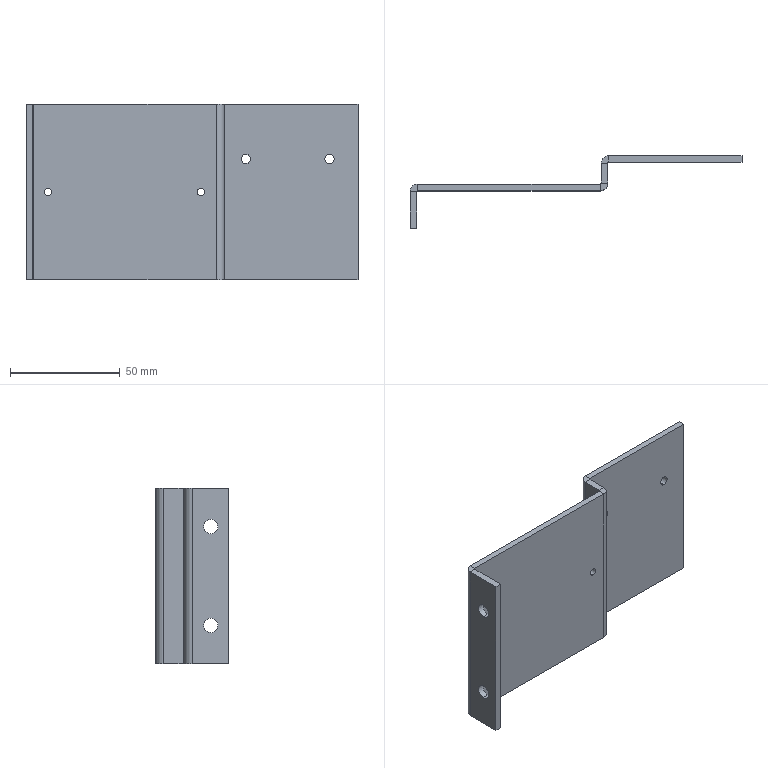Part | SolidWorks | features EdgeFlange 3, HoleWzd 3, FlatPattern 1, SMBaseFlange 1, SheetMetal 1 | 1 solid | 42 faces | box 151 x 33 x 80 mm | volume 42488 mm3 | plane 24 | cylinder 18 | commonest cylinder face diameters 3.3 x4 4.2 x4 6.5 x4 1 x3 7 x3
STEP:
#1=CARTESIAN_POINT('',(55.,13.,17.1));
#2=VERTEX_POINT('',#1);
#3=CARTESIAN_POINT('',(55.,13.,12.9));
#4=VERTEX_POINT('',#3);
#5=CARTESIAN_POINT('',(55.,13.,15.));
#6=DIRECTION('',(0.,-1.,0.));
#7=DIRECTION('',(0.,0.,-1.));
#8=AXIS2_PLACEMENT_3D('',#5,#6,#7);
#9=CIRCLE('',#8,2.1);
#10=EDGE_CURVE('',#2,#4,#9,.T.);
#11=ORIENTED_EDGE('',*,*,#10,.F.);
#12=CARTESIAN_POINT('',(55.,10.,17.1));
#13=VERTEX_POINT('',#12);
#14=CARTESIAN_POINT('',(55.,10.,17.1));
#15=DIRECTION('',(0.,-1.,0.));
#16=VECTOR('',#15,1000.);
#17=LINE('',#14,#16);
#18=EDGE_CURVE('',#2,#13,#17,.T.);
#19=ORIENTED_EDGE('',*,*,#18,.T.);
#20=CARTESIAN_POINT('',(55.,10.,12.9));
#21=VERTEX_POINT('',#20);
#22=CARTESIAN_POINT('',(55.,10.,15.));
#23=DIRECTION('',(0.,-1.,0.));
#24=DIRECTION('',(0.,0.,-1.));
#25=AXIS2_PLACEMENT_3D('',#22,#23,#24);
#26=CIRCLE('',#25,2.1);
#27=EDGE_CURVE('',#13,#21,#26,.T.);
#28=ORIENTED_EDGE('',*,*,#27,.T.);
#29=CARTESIAN_POINT('',(55.,10.,12.9));
#30=DIRECTION('',(0.,-1.,0.));
#31=VECTOR('',#30,1000.);
#32=LINE('',#29,#31);
#33=EDGE_CURVE('',#4,#21,#32,.T.);
#34=ORIENTED_EDGE('',*,*,#33,.F.);
#35=EDGE_LOOP('',(#11,#19,#28,#34));
#36=FACE_OUTER_BOUND('',#35,.T.);
#37=CARTESIAN_POINT('',(55.,10.,15.));
#38=DIRECTION('',(0.,-1.,0.));
#39=DIRECTION('',(0.,0.,-1.));
#40=AXIS2_PLACEMENT_3D('',#37,#38,#39);
#41=CYLINDRICAL_SURFACE('',#40,2.1);
#42=ADVANCED_FACE('',(#36),#41,.F.);
#43=CARTESIAN_POINT('',(93.,13.,17.1));
#44=VERTEX_POINT('',#43);
#45=CARTESIAN_POINT('',(93.,13.,12.9));
#46=VERTEX_POINT('',#45);
#47=CARTESIAN_POINT('',(93.,13.,15.));
#48=DIRECTION('',(0.,-1.,0.));
#49=DIRECTION('',(0.,0.,-1.));
#50=AXIS2_PLACEMENT_3D('',#47,#48,#49);
#51=CIRCLE('',#50,2.1);
#52=EDGE_CURVE('',#44,#46,#51,.T.);
#53=ORIENTED_EDGE('',*,*,#52,.F.);
#54=CARTESIAN_POINT('',(93.,10.,17.1));
#55=VERTEX_POINT('',#54);
#56=CARTESIAN_POINT('',(93.,10.,17.1));
#57=DIRECTION('',(0.,-1.,0.));
#58=VECTOR('',#57,1000.);
#59=LINE('',#56,#58);
#60=EDGE_CURVE('',#44,#55,#59,.T.);
#61=ORIENTED_EDGE('',*,*,#60,.T.);
#62=CARTESIAN_POINT('',(93.,10.,12.9));
#63=VERTEX_POINT('',#62);
#64=CARTESIAN_POINT('',(93.,10.,15.));
#65=DIRECTION('',(0.,-1.,0.));
#66=DIRECTION('',(0.,0.,-1.));
#67=AXIS2_PLACEMENT_3D('',#64,#65,#66);
#68=CIRCLE('',#67,2.1);
#69=EDGE_CURVE('',#55,#63,#68,.T.);
#70=ORIENTED_EDGE('',*,*,#69,.T.);
#71=CARTESIAN_POINT('',(93.,10.,12.9));
#72=DIRECTION('',(0.,-1.,0.));
#73=VECTOR('',#72,1000.);
#74=LINE('',#71,#73);
#75=EDGE_CURVE('',#46,#63,#74,.T.);
#76=ORIENTED_EDGE('',*,*,#75,.F.);
#77=EDGE_LOOP('',(#53,#61,#70,#76));
#78=FACE_OUTER_BOUND('',#77,.T.);
#79=CARTESIAN_POINT('',(93.,10.,15.));
#80=DIRECTION('',(0.,-1.,0.));
#81=DIRECTION('',(0.,0.,-1.));
#82=AXIS2_PLACEMENT_3D('',#79,#80,#81);
#83=CYLINDRICAL_SURFACE('',#82,2.1);
#84=ADVANCED_FACE('',(#78),#83,.F.);
#85=CARTESIAN_POINT('',(-45.,-12.,25.75));
#86=VERTEX_POINT('',#85);
#87=CARTESIAN_POINT('',(-45.,-12.,19.25));
#88=VERTEX_POINT('',#87);
#89=CARTESIAN_POINT('',(-45.,-12.,22.5));
#90=DIRECTION('',(1.,0.,0.));
#91=DIRECTION('',(0.,0.,-1.));
#92=AXIS2_PLACEMENT_3D('',#89,#90,#91);
#93=CIRCLE('',#92,3.25);
#94=EDGE_CURVE('',#86,#88,#93,.T.);
#95=ORIENTED_EDGE('',*,*,#94,.F.);
#96=CARTESIAN_POINT('',(-42.,-12.,25.75));
#97=VERTEX_POINT('',#96);
#98=CARTESIAN_POINT('',(-42.,-12.,25.75));
#99=DIRECTION('',(1.,0.,0.));
#100=VECTOR('',#99,1000.);
#101=LINE('',#98,#100);
#102=EDGE_CURVE('',#86,#97,#101,.T.);
#103=ORIENTED_EDGE('',*,*,#102,.T.);
#104=CARTESIAN_POINT('',(-42.,-12.,19.25));
#105=VERTEX_POINT('',#104);
#106=CARTESIAN_POINT('',(-42.,-12.,22.5));
#107=DIRECTION('',(1.,0.,0.));
#108=DIRECTION('',(0.,0.,-1.));
#109=AXIS2_PLACEMENT_3D('',#106,#107,#108);
#110=CIRCLE('',#109,3.25);
#111=EDGE_CURVE('',#97,#105,#110,.T.);
#112=ORIENTED_EDGE('',*,*,#111,.T.);
#113=CARTESIAN_POINT('',(-42.,-12.,19.25));
#114=DIRECTION('',(1.,0.,0.));
#115=VECTOR('',#114,1000.);
#116=LINE('',#113,#115);
#117=EDGE_CURVE('',#88,#105,#116,.T.);
#118=ORIENTED_EDGE('',*,*,#117,.F.);
#119=EDGE_LOOP('',(#95,#103,#112,#118));
#120=FACE_OUTER_BOUND('',#119,.T.);
#121=CARTESIAN_POINT('',(-42.,-12.,22.5));
#122=DIRECTION('',(1.,0.,0.));
#123=DIRECTION('',(0.,0.,-1.));
#124=AXIS2_PLACEMENT_3D('',#121,#122,#123);
#125=CYLINDRICAL_SURFACE('',#124,3.25);
#126=ADVANCED_FACE('',(#120),#125,.F.);
#127=CARTESIAN_POINT('',(-45.,-12.,-19.25));
#128=VERTEX_POINT('',#127);
#129=CARTESIAN_POINT('',(-45.,-12.,-25.75));
#130=VERTEX_POINT('',#129);
#131=CARTESIAN_POINT('',(-45.,-12.,-22.5));
#132=DIRECTION('',(1.,0.,0.));
#133=DIRECTION('',(0.,0.,-1.));
#134=AXIS2_PLACEMENT_3D('',#131,#132,#133);
#135=CIRCLE('',#134,3.25);
#136=EDGE_CURVE('',#128,#130,#135,.T.);
#137=ORIENTED_EDGE('',*,*,#136,.F.);
#138=CARTESIAN_POINT('',(-42.,-12.,-19.25));
#139=VERTEX_POINT('',#138);
#140=CARTESIAN_POINT('',(-42.,-12.,-19.25));
#141=DIRECTION('',(1.,0.,0.));
#142=VECTOR('',#141,1000.);
#143=LINE('',#140,#142);
#144=EDGE_CURVE('',#128,#139,#143,.T.);
#145=ORIENTED_EDGE('',*,*,#144,.T.);
#146=CARTESIAN_POINT('',(-42.,-12.,-25.75));
#147=VERTEX_POINT('',#146);
#148=CARTESIAN_POINT('',(-42.,-12.,-22.5));
#149=DIRECTION('',(1.,0.,0.));
#150=DIRECTION('',(0.,0.,-1.));
#151=AXIS2_PLACEMENT_3D('',#148,#149,#150);
#152=CIRCLE('',#151,3.25);
#153=EDGE_CURVE('',#139,#147,#152,.T.);
#154=ORIENTED_EDGE('',*,*,#153,.T.);
#155=CARTESIAN_POINT('',(-42.,-12.,-25.75));
#156=DIRECTION('',(1.,0.,0.));
#157=VECTOR('',#156,1000.);
#158=LINE('',#155,#157);
#159=EDGE_CURVE('',#130,#147,#158,.T.);
#160=ORIENTED_EDGE('',*,*,#159,.F.);
#161=EDGE_LOOP('',(#137,#145,#154,#160));
#162=FACE_OUTER_BOUND('',#161,.T.);
#163=CARTESIAN_POINT('',(-42.,-12.,-22.5));
#164=DIRECTION('',(1.,0.,0.));
#165=DIRECTION('',(0.,0.,-1.));
#166=AXIS2_PLACEMENT_3D('',#163,#164,#165);
#167=CYLINDRICAL_SURFACE('',#166,3.25);
#168=ADVANCED_FACE('',(#162),#167,.F.);
#169=CARTESIAN_POINT('',(-35.,-3.,-1.65));
#170=VERTEX_POINT('',#169);
#171=CARTESIAN_POINT('',(-35.,-3.,1.65));
#172=VERTEX_POINT('',#171);
#173=CARTESIAN_POINT('',(-35.,-3.,0.));
#174=DIRECTION('',(0.,1.,0.));
#175=DIRECTION('',(0.,0.,1.));
#176=AXIS2_PLACEMENT_3D('',#173,#174,#175);
#177=CIRCLE('',#176,1.65);
#178=EDGE_CURVE('',#170,#172,#177,.T.);
#179=ORIENTED_EDGE('',*,*,#178,.F.);
#180=CARTESIAN_POINT('',(-35.,0.,-1.65));
#181=VERTEX_POINT('',#180);
#182=CARTESIAN_POINT('',(-35.,0.,-1.65));
#183=DIRECTION('',(0.,1.,0.));
#184=VECTOR('',#183,1000.);
#185=LINE('',#182,#184);
#186=EDGE_CURVE('',#170,#181,#185,.T.);
#187=ORIENTED_EDGE('',*,*,#186,.T.);
#188=CARTESIAN_POINT('',(-35.,0.,1.65));
#189=VERTEX_POINT('',#188);
#190=CARTESIAN_POINT('',(-35.,0.,0.));
#191=DIRECTION('',(0.,1.,0.));
#192=DIRECTION('',(0.,0.,1.));
#193=AXIS2_PLACEMENT_3D('',#190,#191,#192);
#194=CIRCLE('',#193,1.65);
#195=EDGE_CURVE('',#181,#189,#194,.T.);
#196=ORIENTED_EDGE('',*,*,#195,.T.);
#197=CARTESIAN_POINT('',(-35.,0.,1.65));
#198=DIRECTION('',(0.,1.,0.));
#199=VECTOR('',#198,1000.);
#200=LINE('',#197,#199);
#201=EDGE_CURVE('',#172,#189,#200,.T.);
#202=ORIENTED_EDGE('',*,*,#201,.F.);
#203=EDGE_LOOP('',(#179,#187,#196,#202));
#204=FACE_OUTER_BOUND('',#203,.T.);
#205=CARTESIAN_POINT('',(-35.,0.,0.));
#206=DIRECTION('',(0.,1.,0.));
#207=DIRECTION('',(0.,0.,1.));
#208=AXIS2_PLACEMENT_3D('',#205,#206,#207);
#209=CYLINDRICAL_SURFACE('',#208,1.65);
#210=ADVANCED_FACE('',(#204),#209,.F.);
#211=CARTESIAN_POINT('',(34.46,-3.,-1.65));
#212=VERTEX_POINT('',#211);
#213=CARTESIAN_POINT('',(34.46,-3.,1.65));
#214=VERTEX_POINT('',#213);
#215=CARTESIAN_POINT('',(34.46,-3.,0.));
#216=DIRECTION('',(0.,1.,0.));
#217=DIRECTION('',(0.,0.,1.));
#218=AXIS2_PLACEMENT_3D('',#215,#216,#217);
#219=CIRCLE('',#218,1.65);
#220=EDGE_CURVE('',#212,#214,#219,.T.);
#221=ORIENTED_EDGE('',*,*,#220,.F.);
#222=CARTESIAN_POINT('',(34.46,0.,-1.65));
#223=VERTEX_POINT('',#222);
#224=CARTESIAN_POINT('',(34.46,0.,-1.65));
#225=DIRECTION('',(0.,1.,0.));
#226=VECTOR('',#225,1000.);
#227=LINE('',#224,#226);
#228=EDGE_CURVE('',#212,#223,#227,.T.);
#229=ORIENTED_EDGE('',*,*,#228,.T.);
#230=CARTESIAN_POINT('',(34.46,0.,1.65));
#231=VERTEX_POINT('',#230);
#232=CARTESIAN_POINT('',(34.46,0.,0.));
#233=DIRECTION('',(0.,1.,0.));
#234=DIRECTION('',(0.,0.,1.));
#235=AXIS2_PLACEMENT_3D('',#232,#233,#234);
#236=CIRCLE('',#235,1.65);
#237=EDGE_CURVE('',#223,#231,#236,.T.);
#238=ORIENTED_EDGE('',*,*,#237,.T.);
#239=CARTESIAN_POINT('',(34.46,0.,1.65));
#240=DIRECTION('',(0.,1.,0.));
#241=VECTOR('',#240,1000.);
#242=LINE('',#239,#241);
#243=EDGE_CURVE('',#214,#231,#242,.T.);
#244=ORIENTED_EDGE('',*,*,#243,.F.);
#245=EDGE_LOOP('',(#221,#229,#238,#244));
#246=FACE_OUTER_BOUND('',#245,.T.);
#247=CARTESIAN_POINT('',(34.46,0.,0.));
#248=DIRECTION('',(0.,1.,0.));
#249=DIRECTION('',(0.,0.,1.));
#250=AXIS2_PLACEMENT_3D('',#247,#248,#249);
#251=CYLINDRICAL_SURFACE('',#250,1.65);
#252=ADVANCED_FACE('',(#246),#251,.F.);
#253=CARTESIAN_POINT('',(34.46,-3.,0.));
#254=DIRECTION('',(0.,1.,0.));
#255=DIRECTION('',(0.,0.,1.));
#256=AXIS2_PLACEMENT_3D('',#253,#254,#255);
#257=CIRCLE('',#256,1.65);
#258=EDGE_CURVE('',#214,#212,#257,.T.);
#259=ORIENTED_EDGE('',*,*,#258,.T.);
#260=ORIENTED_EDGE('',*,*,#220,.T.);
#261=EDGE_LOOP('',(#259,#260));
#262=FACE_BOUND('',#261,.T.);
#263=CARTESIAN_POINT('',(-35.,-3.,0.));
#264=DIRECTION('',(0.,1.,0.));
#265=DIRECTION('',(0.,0.,1.));
#266=AXIS2_PLACEMENT_3D('',#263,#264,#265);
#267=CIRCLE('',#266,1.65);
#268=EDGE_CURVE('',#172,#170,#267,.T.);
#269=ORIENTED_EDGE('',*,*,#268,.T.);
#270=ORIENTED_EDGE('',*,*,#178,.T.);
#271=EDGE_LOOP('',(#269,#270));
#272=FACE_BOUND('',#271,.T.);
#273=CARTESIAN_POINT('',(-41.5,-3.,-40.));
#274=VERTEX_POINT('',#273);
#275=CARTESIAN_POINT('',(-41.5,-3.,40.));
#276=VERTEX_POINT('',#275);
#277=CARTESIAN_POINT('',(-41.5,-3.,-40.));
#278=DIRECTION('',(0.,0.,1.));
#279=VECTOR('',#278,1000.);
#280=LINE('',#277,#279);
#281=EDGE_CURVE('',#274,#276,#280,.T.);
#282=ORIENTED_EDGE('',*,*,#281,.F.);
#283=CARTESIAN_POINT('',(41.5,-3.,-40.));
#284=VERTEX_POINT('',#283);
#285=CARTESIAN_POINT('',(-45.,-3.,-40.));
#286=DIRECTION('',(1.,0.,0.));
#287=VECTOR('',#286,1000.);
#288=LINE('',#285,#287);
#289=EDGE_CURVE('',#274,#284,#288,.T.);
#290=ORIENTED_EDGE('',*,*,#289,.T.);
#291=CARTESIAN_POINT('',(41.5,-3.,40.));
#292=VERTEX_POINT('',#291);
#293=CARTESIAN_POINT('',(41.5,-3.,-40.));
#294=DIRECTION('',(0.,0.,1.));
#295=VECTOR('',#294,1000.);
#296=LINE('',#293,#295);
#297=EDGE_CURVE('',#284,#292,#296,.T.);
#298=ORIENTED_EDGE('',*,*,#297,.T.);
#299=CARTESIAN_POINT('',(-45.,-3.,40.));
#300=DIRECTION('',(1.,0.,0.));
#301=VECTOR('',#300,1000.);
#302=LINE('',#299,#301);
#303=EDGE_CURVE('',#276,#292,#302,.T.);
#304=ORIENTED_EDGE('',*,*,#303,.F.);
#305=EDGE_LOOP('',(#282,#290,#298,#304));
#306=FACE_OUTER_BOUND('',#305,.T.);
#307=CARTESIAN_POINT('',(-45.,-3.,40.));
#308=DIRECTION('',(0.,1.,0.));
#309=DIRECTION('',(-1.,0.,0.));
#310=AXIS2_PLACEMENT_3D('',#307,#308,#309);
#311=PLANE('',#310);
#312=ADVANCED_FACE('',(#262,#272,#306),#311,.F.);
#313=CARTESIAN_POINT('',(-35.,0.,0.));
#314=DIRECTION('',(0.,1.,0.));
#315=DIRECTION('',(0.,0.,1.));
#316=AXIS2_PLACEMENT_3D('',#313,#314,#315);
#317=CIRCLE('',#316,1.65);
#318=EDGE_CURVE('',#189,#181,#317,.T.);
#319=ORIENTED_EDGE('',*,*,#318,.F.);
#320=ORIENTED_EDGE('',*,*,#195,.F.);
#321=EDGE_LOOP('',(#319,#320));
#322=FACE_BOUND('',#321,.T.);
#323=CARTESIAN_POINT('',(34.46,0.,0.));
#324=DIRECTION('',(0.,1.,0.));
#325=DIRECTION('',(0.,0.,1.));
#326=AXIS2_PLACEMENT_3D('',#323,#324,#325);
#327=CIRCLE('',#326,1.65);
#328=EDGE_CURVE('',#231,#223,#327,.T.);
#329=ORIENTED_EDGE('',*,*,#328,.F.);
#330=ORIENTED_EDGE('',*,*,#237,.F.);
#331=EDGE_LOOP('',(#329,#330));
#332=FACE_BOUND('',#331,.T.);
#333=CARTESIAN_POINT('',(-41.5,0.,-40.));
#334=VERTEX_POINT('',#333);
#335=CARTESIAN_POINT('',(41.5,0.,-40.));
#336=VERTEX_POINT('',#335);
#337=CARTESIAN_POINT('',(-45.,0.,-40.));
#338=DIRECTION('',(1.,0.,0.));
#339=VECTOR('',#338,1000.);
#340=LINE('',#337,#339);
#341=EDGE_CURVE('',#334,#336,#340,.T.);
#342=ORIENTED_EDGE('',*,*,#341,.F.);
#343=CARTESIAN_POINT('',(-41.5,0.,40.));
#344=VERTEX_POINT('',#343);
#345=CARTESIAN_POINT('',(-41.5,0.,-40.));
#346=DIRECTION('',(0.,0.,1.));
#347=VECTOR('',#346,1000.);
#348=LINE('',#345,#347);
#349=EDGE_CURVE('',#334,#344,#348,.T.);
#350=ORIENTED_EDGE('',*,*,#349,.T.);
#351=CARTESIAN_POINT('',(41.5,0.,40.));
#352=VERTEX_POINT('',#351);
#353=CARTESIAN_POINT('',(-45.,0.,40.));
#354=DIRECTION('',(1.,0.,0.));
#355=VECTOR('',#354,1000.);
#356=LINE('',#353,#355);
#357=EDGE_CURVE('',#344,#352,#356,.T.);
#358=ORIENTED_EDGE('',*,*,#357,.T.);
#359=CARTESIAN_POINT('',(41.5,0.,-40.));
#360=DIRECTION('',(0.,0.,1.));
#361=VECTOR('',#360,1000.);
#362=LINE('',#359,#361);
#363=EDGE_CURVE('',#336,#352,#362,.T.);
#364=ORIENTED_EDGE('',*,*,#363,.F.);
#365=EDGE_LOOP('',(#342,#350,#358,#364));
#366=FACE_OUTER_BOUND('',#365,.T.);
#367=CARTESIAN_POINT('',(-45.,0.,40.));
#368=DIRECTION('',(0.,1.,0.));
#369=DIRECTION('',(-1.,0.,0.));
#370=AXIS2_PLACEMENT_3D('',#367,#368,#369);
#371=PLANE('',#370);
#372=ADVANCED_FACE('',(#322,#332,#366),#371,.T.);
#373=CARTESIAN_POINT('',(-41.5,-3.,40.));
#374=DIRECTION('',(0.,1.,0.));
#375=VECTOR('',#374,1000.);
#376=LINE('',#373,#375);
#377=EDGE_CURVE('',#276,#344,#376,.T.);
#378=ORIENTED_EDGE('',*,*,#377,.F.);
#379=ORIENTED_EDGE('',*,*,#303,.T.);
#380=CARTESIAN_POINT('',(41.5,0.,40.));
#381=DIRECTION('',(0.,-1.,0.));
#382=VECTOR('',#381,1000.);
#383=LINE('',#380,#382);
#384=EDGE_CURVE('',#352,#292,#383,.T.);
#385=ORIENTED_EDGE('',*,*,#384,.F.);
#386=ORIENTED_EDGE('',*,*,#357,.F.);
#387=EDGE_LOOP('',(#378,#379,#385,#386));
#388=FACE_OUTER_BOUND('',#387,.T.);
#389=CARTESIAN_POINT('',(0.,0.,40.));
#390=DIRECTION('',(0.,0.,-1.));
#391=DIRECTION('',(-1.,0.,0.));
#392=AXIS2_PLACEMENT_3D('',#389,#390,#391);
#393=PLANE('',#392);
#394=ADVANCED_FACE('',(#388),#393,.F.);
#395=ORIENTED_EDGE('',*,*,#289,.F.);
#396=CARTESIAN_POINT('',(-41.5,-3.,-40.));
#397=DIRECTION('',(0.,1.,0.));
#398=VECTOR('',#397,1000.);
#399=LINE('',#396,#398);
#400=EDGE_CURVE('',#274,#334,#399,.T.);
#401=ORIENTED_EDGE('',*,*,#400,.T.);
#402=ORIENTED_EDGE('',*,*,#341,.T.);
#403=CARTESIAN_POINT('',(41.5,0.,-40.));
#404=DIRECTION('',(0.,-1.,0.));
#405=VECTOR('',#404,1000.);
#406=LINE('',#403,#405);
#407=EDGE_CURVE('',#336,#284,#406,.T.);
#408=ORIENTED_EDGE('',*,*,#407,.T.);
#409=EDGE_LOOP('',(#395,#401,#402,#408));
#410=FACE_OUTER_BOUND('',#409,.T.);
#411=CARTESIAN_POINT('',(0.,0.,-40.));
#412=DIRECTION('',(0.,0.,-1.));
#413=DIRECTION('',(-1.,0.,0.));
#414=AXIS2_PLACEMENT_3D('',#411,#412,#413);
#415=PLANE('',#414);
#416=ADVANCED_FACE('',(#410),#415,.T.);
#417=CARTESIAN_POINT('',(45.,9.5,40.));
#418=VERTEX_POINT('',#417);
#419=CARTESIAN_POINT('',(42.,9.5,40.));
#420=VERTEX_POINT('',#419);
#421=CARTESIAN_POINT('',(45.,9.5,40.));
#422=DIRECTION('',(-1.,0.,0.));
#423=VECTOR('',#422,1000.);
#424=LINE('',#421,#423);
#425=EDGE_CURVE('',#418,#420,#424,.T.);
#426=ORIENTED_EDGE('',*,*,#425,.T.);
#427=CARTESIAN_POINT('',(42.,0.5,40.));
#428=VERTEX_POINT('',#427);
#429=CARTESIAN_POINT('',(42.,0.,40.));
#430=DIRECTION('',(0.,-1.,0.));
#431=VECTOR('',#430,1000.);
#432=LINE('',#429,#431);
#433=EDGE_CURVE('',#420,#428,#432,.T.);
#434=ORIENTED_EDGE('',*,*,#433,.T.);
#435=CARTESIAN_POINT('',(45.,0.5,40.));
#436=VERTEX_POINT('',#435);
#437=CARTESIAN_POINT('',(45.,0.5,40.));
#438=DIRECTION('',(1.,0.,0.));
#439=VECTOR('',#438,1000.);
#440=LINE('',#437,#439);
#441=EDGE_CURVE('',#428,#436,#440,.T.);
#442=ORIENTED_EDGE('',*,*,#441,.T.);
#443=CARTESIAN_POINT('',(45.,0.,40.));
#444=DIRECTION('',(0.,-1.,0.));
#445=VECTOR('',#444,1000.);
#446=LINE('',#443,#445);
#447=EDGE_CURVE('',#418,#436,#446,.T.);
#448=ORIENTED_EDGE('',*,*,#447,.F.);
#449=EDGE_LOOP('',(#426,#434,#442,#448));
#450=FACE_OUTER_BOUND('',#449,.T.);
#451=CARTESIAN_POINT('',(45.,0.,40.));
#452=DIRECTION('',(0.,0.,-1.));
#453=DIRECTION('',(-1.,0.,0.));
#454=AXIS2_PLACEMENT_3D('',#451,#452,#453);
#455=PLANE('',#454);
#456=ADVANCED_FACE('',(#450),#455,.F.);
#457=CARTESIAN_POINT('',(45.,9.5,-40.));
#458=VERTEX_POINT('',#457);
#459=CARTESIAN_POINT('',(42.,9.5,-40.));
#460=VERTEX_POINT('',#459);
#461=CARTESIAN_POINT('',(45.,9.5,-40.));
#462=DIRECTION('',(-1.,0.,0.));
#463=VECTOR('',#462,1000.);
#464=LINE('',#461,#463);
#465=EDGE_CURVE('',#458,#460,#464,.T.);
#466=ORIENTED_EDGE('',*,*,#465,.F.);
#467=CARTESIAN_POINT('',(45.,0.5,-40.));
#468=VERTEX_POINT('',#467);
#469=CARTESIAN_POINT('',(45.,0.,-40.));
#470=DIRECTION('',(0.,1.,0.));
#471=VECTOR('',#470,1000.);
#472=LINE('',#469,#471);
#473=EDGE_CURVE('',#468,#458,#472,.T.);
#474=ORIENTED_EDGE('',*,*,#473,.F.);
#475=CARTESIAN_POINT('',(42.,0.5,-40.));
#476=VERTEX_POINT('',#475);
#477=CARTESIAN_POINT('',(42.,0.5,-40.));
#478=DIRECTION('',(1.,0.,0.));
#479=VECTOR('',#478,1000.);
#480=LINE('',#477,#479);
#481=EDGE_CURVE('',#476,#468,#480,.T.);
#482=ORIENTED_EDGE('',*,*,#481,.F.);
#483=CARTESIAN_POINT('',(42.,13.,-40.));
#484=DIRECTION('',(0.,1.,0.));
#485=VECTOR('',#484,1000.);
#486=LINE('',#483,#485);
#487=EDGE_CURVE('',#476,#460,#486,.T.);
#488=ORIENTED_EDGE('',*,*,#487,.T.);
#489=EDGE_LOOP('',(#466,#474,#482,#488));
#490=FACE_OUTER_BOUND('',#489,.T.);
#491=CARTESIAN_POINT('',(45.,13.,-40.));
#492=DIRECTION('',(0.,0.,1.));
#493=DIRECTION('',(0.,-1.,0.));
#494=AXIS2_PLACEMENT_3D('',#491,#492,#493);
#495=PLANE('',#494);
#496=ADVANCED_FACE('',(#490),#495,.F.);
#497=CARTESIAN_POINT('',(45.,9.5,40.));
#498=DIRECTION('',(0.,0.,-1.));
#499=VECTOR('',#498,1000.);
#500=LINE('',#497,#499);
#501=EDGE_CURVE('',#418,#458,#500,.T.);
#502=ORIENTED_EDGE('',*,*,#501,.F.);
#503=ORIENTED_EDGE('',*,*,#447,.T.);
#504=CARTESIAN_POINT('',(45.,0.5,40.));
#505=DIRECTION('',(0.,0.,1.));
#506=VECTOR('',#505,1000.);
#507=LINE('',#504,#506);
#508=EDGE_CURVE('',#468,#436,#507,.T.);
#509=ORIENTED_EDGE('',*,*,#508,.F.);
#510=ORIENTED_EDGE('',*,*,#473,.T.);
#511=EDGE_LOOP('',(#502,#503,#509,#510));
#512=FACE_OUTER_BOUND('',#511,.T.);
#513=CARTESIAN_POINT('',(45.,0.,0.));
#514=DIRECTION('',(-1.,0.,0.));
#515=DIRECTION('',(0.,-1.,0.));
#516=AXIS2_PLACEMENT_3D('',#513,#514,#515);
#517=PLANE('',#516);
#518=ADVANCED_FACE('',(#512),#517,.F.);
#519=ORIENTED_EDGE('',*,*,#433,.F.);
#520=CARTESIAN_POINT('',(42.,9.5,40.));
#521=DIRECTION('',(0.,0.,-1.));
#522=VECTOR('',#521,1000.);
#523=LINE('',#520,#522);
#524=EDGE_CURVE('',#420,#460,#523,.T.);
#525=ORIENTED_EDGE('',*,*,#524,.T.);
#526=ORIENTED_EDGE('',*,*,#487,.F.);
#527=CARTESIAN_POINT('',(42.,0.5,40.));
#528=DIRECTION('',(0.,0.,-1.));
#529=VECTOR('',#528,1000.);
#530=LINE('',#527,#529);
#531=EDGE_CURVE('',#428,#476,#530,.T.);
#532=ORIENTED_EDGE('',*,*,#531,.F.);
#533=EDGE_LOOP('',(#519,#525,#526,#532));
#534=FACE_OUTER_BOUND('',#533,.T.);
#535=CARTESIAN_POINT('',(42.,0.,0.));
#536=DIRECTION('',(-1.,0.,0.));
#537=DIRECTION('',(0.,-1.,0.));
#538=AXIS2_PLACEMENT_3D('',#535,#536,#537);
#539=PLANE('',#538);
#540=ADVANCED_FACE('',(#534),#539,.T.);
#541=ORIENTED_EDGE('',*,*,#441,.F.);
#542=CARTESIAN_POINT('',(41.5,0.5,40.));
#543=DIRECTION('',(0.,0.,1.));
#544=DIRECTION('',(-1.,0.,0.));
#545=AXIS2_PLACEMENT_3D('',#542,#543,#544);
#546=CIRCLE('',#545,0.5);
#547=EDGE_CURVE('',#352,#428,#546,.T.);
#548=ORIENTED_EDGE('',*,*,#547,.F.);
#549=ORIENTED_EDGE('',*,*,#384,.T.);
#550=CARTESIAN_POINT('',(41.5,0.5,40.));
#551=DIRECTION('',(0.,0.,1.));
#552=DIRECTION('',(-1.,0.,0.));
#553=AXIS2_PLACEMENT_3D('',#550,#551,#552);
#554=CIRCLE('',#553,3.5);
#555=EDGE_CURVE('',#292,#436,#554,.T.);
#556=ORIENTED_EDGE('',*,*,#555,.T.);
#557=EDGE_LOOP('',(#541,#548,#549,#556));
#558=FACE_OUTER_BOUND('',#557,.T.);
#559=CARTESIAN_POINT('',(41.5,0.5,40.));
#560=DIRECTION('',(0.,0.,1.));
#561=DIRECTION('',(1.,0.,0.));
#562=AXIS2_PLACEMENT_3D('',#559,#560,#561);
#563=PLANE('',#562);
#564=ADVANCED_FACE('',(#558),#563,.T.);
#565=CARTESIAN_POINT('',(41.5,0.5,-40.));
#566=DIRECTION('',(0.,0.,-1.));
#567=DIRECTION('',(-1.,0.,0.));
#568=AXIS2_PLACEMENT_3D('',#565,#566,#567);
#569=CIRCLE('',#568,0.5);
#570=EDGE_CURVE('',#476,#336,#569,.T.);
#571=ORIENTED_EDGE('',*,*,#570,.F.);
#572=ORIENTED_EDGE('',*,*,#481,.T.);
#573=CARTESIAN_POINT('',(41.5,0.5,-40.));
#574=DIRECTION('',(0.,0.,-1.));
#575=DIRECTION('',(-1.,0.,0.));
#576=AXIS2_PLACEMENT_3D('',#573,#574,#575);
#577=CIRCLE('',#576,3.5);
#578=EDGE_CURVE('',#468,#284,#577,.T.);
#579=ORIENTED_EDGE('',*,*,#578,.T.);
#580=ORIENTED_EDGE('',*,*,#407,.F.);
#581=EDGE_LOOP('',(#571,#572,#579,#580));
#582=FACE_OUTER_BOUND('',#581,.T.);
#583=CARTESIAN_POINT('',(41.5,0.5,-40.));
#584=DIRECTION('',(0.,0.,1.));
#585=DIRECTION('',(1.,0.,0.));
#586=AXIS2_PLACEMENT_3D('',#583,#584,#585);
#587=PLANE('',#586);
#588=ADVANCED_FACE('',(#582),#587,.F.);
#589=ORIENTED_EDGE('',*,*,#297,.F.);
#590=ORIENTED_EDGE('',*,*,#578,.F.);
#591=ORIENTED_EDGE('',*,*,#508,.T.);
#592=ORIENTED_EDGE('',*,*,#555,.F.);
#593=EDGE_LOOP('',(#589,#590,#591,#592));
#594=FACE_OUTER_BOUND('',#593,.T.);
#595=CARTESIAN_POINT('',(41.5,0.5,-40.));
#596=DIRECTION('',(0.,0.,-1.));
#597=DIRECTION('',(1.,0.,0.));
#598=AXIS2_PLACEMENT_3D('',#595,#596,#597);
#599=CYLINDRICAL_SURFACE('',#598,3.5);
#600=ADVANCED_FACE('',(#594),#599,.T.);
#601=ORIENTED_EDGE('',*,*,#363,.T.);
#602=ORIENTED_EDGE('',*,*,#547,.T.);
#603=ORIENTED_EDGE('',*,*,#531,.T.);
#604=ORIENTED_EDGE('',*,*,#570,.T.);
#605=EDGE_LOOP('',(#601,#602,#603,#604));
#606=FACE_OUTER_BOUND('',#605,.T.);
#607=CARTESIAN_POINT('',(41.5,0.5,-40.));
#608=DIRECTION('',(0.,0.,-1.));
#609=DIRECTION('',(1.,0.,0.));
#610=AXIS2_PLACEMENT_3D('',#607,#608,#609);
#611=CYLINDRICAL_SURFACE('',#610,0.5);
#612=ADVANCED_FACE('',(#606),#611,.F.);
#613=CARTESIAN_POINT('',(45.5,10.,-40.));
#614=VERTEX_POINT('',#613);
#615=CARTESIAN_POINT('',(45.5,13.,-40.));
#616=VERTEX_POINT('',#615);
#617=CARTESIAN_POINT('',(45.5,13.,-40.));
#618=DIRECTION('',(0.,1.,0.));
#619=VECTOR('',#618,1000.);
#620=LINE('',#617,#619);
#621=EDGE_CURVE('',#614,#616,#620,.T.);
#622=ORIENTED_EDGE('',*,*,#621,.F.);
#623=CARTESIAN_POINT('',(45.5,9.5,-40.));
#624=DIRECTION('',(0.,0.,-1.));
#625=DIRECTION('',(1.,0.,0.));
#626=AXIS2_PLACEMENT_3D('',#623,#624,#625);
#627=CIRCLE('',#626,0.5);
#628=EDGE_CURVE('',#458,#614,#627,.T.);
#629=ORIENTED_EDGE('',*,*,#628,.F.);
#630=ORIENTED_EDGE('',*,*,#465,.T.);
#631=CARTESIAN_POINT('',(45.5,9.5,-40.));
#632=DIRECTION('',(0.,0.,-1.));
#633=DIRECTION('',(1.,0.,0.));
#634=AXIS2_PLACEMENT_3D('',#631,#632,#633);
#635=CIRCLE('',#634,3.5);
#636=EDGE_CURVE('',#460,#616,#635,.T.);
#637=ORIENTED_EDGE('',*,*,#636,.T.);
#638=EDGE_LOOP('',(#622,#629,#630,#637));
#639=FACE_OUTER_BOUND('',#638,.T.);
#640=CARTESIAN_POINT('',(45.5,9.5,-40.));
#641=DIRECTION('',(0.,0.,-1.));
#642=DIRECTION('',(-1.,0.,0.));
#643=AXIS2_PLACEMENT_3D('',#640,#641,#642);
#644=PLANE('',#643);
#645=ADVANCED_FACE('',(#639),#644,.T.);
#646=CARTESIAN_POINT('',(45.5,10.,40.));
#647=VERTEX_POINT('',#646);
#648=CARTESIAN_POINT('',(45.5,9.5,40.));
#649=DIRECTION('',(0.,0.,1.));
#650=DIRECTION('',(1.,0.,0.));
#651=AXIS2_PLACEMENT_3D('',#648,#649,#650);
#652=CIRCLE('',#651,0.5);
#653=EDGE_CURVE('',#647,#418,#652,.T.);
#654=ORIENTED_EDGE('',*,*,#653,.F.);
#655=CARTESIAN_POINT('',(45.5,13.,40.));
#656=VERTEX_POINT('',#655);
#657=CARTESIAN_POINT('',(45.5,10.,40.));
#658=DIRECTION('',(0.,1.,0.));
#659=VECTOR('',#658,1000.);
#660=LINE('',#657,#659);
#661=EDGE_CURVE('',#647,#656,#660,.T.);
#662=ORIENTED_EDGE('',*,*,#661,.T.);
#663=CARTESIAN_POINT('',(45.5,9.5,40.));
#664=DIRECTION('',(0.,0.,1.));
#665=DIRECTION('',(1.,0.,0.));
#666=AXIS2_PLACEMENT_3D('',#663,#664,#665);
#667=CIRCLE('',#666,3.5);
#668=EDGE_CURVE('',#656,#420,#667,.T.);
#669=ORIENTED_EDGE('',*,*,#668,.T.);
#670=ORIENTED_EDGE('',*,*,#425,.F.);
#671=EDGE_LOOP('',(#654,#662,#669,#670));
#672=FACE_OUTER_BOUND('',#671,.T.);
#673=CARTESIAN_POINT('',(45.5,9.5,40.));
#674=DIRECTION('',(0.,0.,-1.));
#675=DIRECTION('',(-1.,0.,0.));
#676=AXIS2_PLACEMENT_3D('',#673,#674,#675);
#677=PLANE('',#676);
#678=ADVANCED_FACE('',(#672),#677,.F.);
#679=ORIENTED_EDGE('',*,*,#524,.F.);
#680=ORIENTED_EDGE('',*,*,#668,.F.);
#681=CARTESIAN_POINT('',(45.5,13.,-40.));
#682=DIRECTION('',(0.,0.,-1.));
#683=VECTOR('',#682,1000.);
#684=LINE('',#681,#683);
#685=EDGE_CURVE('',#656,#616,#684,.T.);
#686=ORIENTED_EDGE('',*,*,#685,.T.);
#687=ORIENTED_EDGE('',*,*,#636,.F.);
#688=EDGE_LOOP('',(#679,#680,#686,#687));
#689=FACE_OUTER_BOUND('',#688,.T.);
#690=CARTESIAN_POINT('',(45.5,9.5,40.));
#691=DIRECTION('',(0.,0.,1.));
#692=DIRECTION('',(0.,1.,0.));
#693=AXIS2_PLACEMENT_3D('',#690,#691,#692);
#694=CYLINDRICAL_SURFACE('',#693,3.5);
#695=ADVANCED_FACE('',(#689),#694,.T.);
#696=ORIENTED_EDGE('',*,*,#501,.T.);
#697=ORIENTED_EDGE('',*,*,#628,.T.);
#698=CARTESIAN_POINT('',(45.5,10.,-40.));
#699=DIRECTION('',(0.,0.,1.));
#700=VECTOR('',#699,1000.);
#701=LINE('',#698,#700);
#702=EDGE_CURVE('',#614,#647,#701,.T.);
#703=ORIENTED_EDGE('',*,*,#702,.T.);
#704=ORIENTED_EDGE('',*,*,#653,.T.);
#705=EDGE_LOOP('',(#696,#697,#703,#704));
#706=FACE_OUTER_BOUND('',#705,.T.);
#707=CARTESIAN_POINT('',(45.5,9.5,40.));
#708=DIRECTION('',(0.,0.,1.));
#709=DIRECTION('',(0.,1.,0.));
#710=AXIS2_PLACEMENT_3D('',#707,#708,#709);
#711=CYLINDRICAL_SURFACE('',#710,0.5);
#712=ADVANCED_FACE('',(#706),#711,.F.);
#713=ORIENTED_EDGE('',*,*,#621,.T.);
#714=CARTESIAN_POINT('',(106.,13.,-40.));
#715=VERTEX_POINT('',#714);
#716=CARTESIAN_POINT('',(0.,13.,-40.));
#717=DIRECTION('',(-1.,0.,0.));
#718=VECTOR('',#717,1000.);
#719=LINE('',#716,#718);
#720=EDGE_CURVE('',#715,#616,#719,.T.);
#721=ORIENTED_EDGE('',*,*,#720,.F.);
#722=CARTESIAN_POINT('',(106.,10.,-40.));
#723=VERTEX_POINT('',#722);
#724=CARTESIAN_POINT('',(106.,13.,-40.));
#725=DIRECTION('',(0.,-1.,0.));
#726=VECTOR('',#725,1000.);
#727=LINE('',#724,#726);
#728=EDGE_CURVE('',#715,#723,#727,.T.);
#729=ORIENTED_EDGE('',*,*,#728,.T.);
#730=CARTESIAN_POINT('',(45.,10.,-40.));
#731=DIRECTION('',(-1.,0.,0.));
#732=VECTOR('',#731,1000.);
#733=LINE('',#730,#732);
#734=EDGE_CURVE('',#723,#614,#733,.T.);
#735=ORIENTED_EDGE('',*,*,#734,.T.);
#736=EDGE_LOOP('',(#713,#721,#729,#735));
#737=FACE_OUTER_BOUND('',#736,.T.);
#738=CARTESIAN_POINT('',(45.,13.,-40.));
#739=DIRECTION('',(0.,0.,1.));
#740=DIRECTION('',(1.,0.,0.));
#741=AXIS2_PLACEMENT_3D('',#738,#739,#740);
#742=PLANE('',#741);
#743=ADVANCED_FACE('',(#737),#742,.F.);
#744=ORIENTED_EDGE('',*,*,#661,.F.);
#745=CARTESIAN_POINT('',(106.,10.,40.));
#746=VERTEX_POINT('',#745);
#747=CARTESIAN_POINT('',(106.,10.,40.));
#748=DIRECTION('',(1.,0.,0.));
#749=VECTOR('',#748,1000.);
#750=LINE('',#747,#749);
#751=EDGE_CURVE('',#647,#746,#750,.T.);
#752=ORIENTED_EDGE('',*,*,#751,.T.);
#753=CARTESIAN_POINT('',(106.,13.,40.));
#754=VERTEX_POINT('',#753);
#755=CARTESIAN_POINT('',(106.,13.,40.));
#756=DIRECTION('',(0.,-1.,0.));
#757=VECTOR('',#756,1000.);
#758=LINE('',#755,#757);
#759=EDGE_CURVE('',#754,#746,#758,.T.);
#760=ORIENTED_EDGE('',*,*,#759,.F.);
#761=CARTESIAN_POINT('',(0.,13.,40.));
#762=DIRECTION('',(1.,0.,0.));
#763=VECTOR('',#762,1000.);
#764=LINE('',#761,#763);
#765=EDGE_CURVE('',#656,#754,#764,.T.);
#766=ORIENTED_EDGE('',*,*,#765,.F.);
#767=EDGE_LOOP('',(#744,#752,#760,#766));
#768=FACE_OUTER_BOUND('',#767,.T.);
#769=CARTESIAN_POINT('',(106.,13.,40.));
#770=DIRECTION('',(0.,0.,-1.));
#771=DIRECTION('',(-1.,0.,0.));
#772=AXIS2_PLACEMENT_3D('',#769,#770,#771);
#773=PLANE('',#772);
#774=ADVANCED_FACE('',(#768),#773,.F.);
#775=CARTESIAN_POINT('',(55.,13.,15.));
#776=DIRECTION('',(0.,-1.,0.));
#777=DIRECTION('',(0.,0.,-1.));
#778=AXIS2_PLACEMENT_3D('',#775,#776,#777);
#779=CIRCLE('',#778,2.1);
#780=EDGE_CURVE('',#4,#2,#779,.T.);
#781=ORIENTED_EDGE('',*,*,#780,.T.);
#782=ORIENTED_EDGE('',*,*,#10,.T.);
#783=EDGE_LOOP('',(#781,#782));
#784=FACE_BOUND('',#783,.T.);
#785=CARTESIAN_POINT('',(93.,13.,15.));
#786=DIRECTION('',(0.,-1.,0.));
#787=DIRECTION('',(0.,0.,-1.));
#788=AXIS2_PLACEMENT_3D('',#785,#786,#787);
#789=CIRCLE('',#788,2.1);
#790=EDGE_CURVE('',#46,#44,#789,.T.);
#791=ORIENTED_EDGE('',*,*,#790,.T.);
#792=ORIENTED_EDGE('',*,*,#52,.T.);
#793=EDGE_LOOP('',(#791,#792));
#794=FACE_BOUND('',#793,.T.);
#795=ORIENTED_EDGE('',*,*,#685,.F.);
#796=ORIENTED_EDGE('',*,*,#765,.T.);
#797=CARTESIAN_POINT('',(106.,13.,0.));
#798=DIRECTION('',(0.,0.,-1.));
#799=VECTOR('',#798,1000.);
#800=LINE('',#797,#799);
#801=EDGE_CURVE('',#754,#715,#800,.T.);
#802=ORIENTED_EDGE('',*,*,#801,.T.);
#803=ORIENTED_EDGE('',*,*,#720,.T.);
#804=EDGE_LOOP('',(#795,#796,#802,#803));
#805=FACE_OUTER_BOUND('',#804,.T.);
#806=CARTESIAN_POINT('',(0.,13.,0.));
#807=DIRECTION('',(0.,-1.,0.));
#808=DIRECTION('',(1.,0.,0.));
#809=AXIS2_PLACEMENT_3D('',#806,#807,#808);
#810=PLANE('',#809);
#811=ADVANCED_FACE('',(#784,#794,#805),#810,.F.);
#812=CARTESIAN_POINT('',(55.,10.,15.));
#813=DIRECTION('',(0.,-1.,0.));
#814=DIRECTION('',(0.,0.,-1.));
#815=AXIS2_PLACEMENT_3D('',#812,#813,#814);
#816=CIRCLE('',#815,2.1);
#817=EDGE_CURVE('',#21,#13,#816,.T.);
#818=ORIENTED_EDGE('',*,*,#817,.F.);
#819=ORIENTED_EDGE('',*,*,#27,.F.);
#820=EDGE_LOOP('',(#818,#819));
#821=FACE_BOUND('',#820,.T.);
#822=CARTESIAN_POINT('',(93.,10.,15.));
#823=DIRECTION('',(0.,-1.,0.));
#824=DIRECTION('',(0.,0.,-1.));
#825=AXIS2_PLACEMENT_3D('',#822,#823,#824);
#826=CIRCLE('',#825,2.1);
#827=EDGE_CURVE('',#63,#55,#826,.T.);
#828=ORIENTED_EDGE('',*,*,#827,.F.);
#829=ORIENTED_EDGE('',*,*,#69,.F.);
#830=EDGE_LOOP('',(#828,#829));
#831=FACE_BOUND('',#830,.T.);
#832=ORIENTED_EDGE('',*,*,#751,.F.);
#833=ORIENTED_EDGE('',*,*,#702,.F.);
#834=ORIENTED_EDGE('',*,*,#734,.F.);
#835=CARTESIAN_POINT('',(106.,10.,-40.));
#836=DIRECTION('',(0.,0.,-1.));
#837=VECTOR('',#836,1000.);
#838=LINE('',#835,#837);
#839=EDGE_CURVE('',#746,#723,#838,.T.);
#840=ORIENTED_EDGE('',*,*,#839,.F.);
#841=EDGE_LOOP('',(#832,#833,#834,#840));
#842=FACE_OUTER_BOUND('',#841,.T.);
#843=CARTESIAN_POINT('',(0.,10.,0.));
#844=DIRECTION('',(0.,-1.,0.));
#845=DIRECTION('',(1.,0.,0.));
#846=AXIS2_PLACEMENT_3D('',#843,#844,#845);
#847=PLANE('',#846);
#848=ADVANCED_FACE('',(#821,#831,#842),#847,.T.);
#849=ORIENTED_EDGE('',*,*,#839,.T.);
#850=ORIENTED_EDGE('',*,*,#728,.F.);
#851=ORIENTED_EDGE('',*,*,#801,.F.);
#852=ORIENTED_EDGE('',*,*,#759,.T.);
#853=EDGE_LOOP('',(#849,#850,#851,#852));
#854=FACE_OUTER_BOUND('',#853,.T.);
#855=CARTESIAN_POINT('',(106.,13.,-40.));
#856=DIRECTION('',(-1.,0.,0.));
#857=DIRECTION('',(0.,-1.,0.));
#858=AXIS2_PLACEMENT_3D('',#855,#856,#857);
#859=PLANE('',#858);
#860=ADVANCED_FACE('',(#854),#859,.F.);
#861=ORIENTED_EDGE('',*,*,#228,.F.);
#862=ORIENTED_EDGE('',*,*,#258,.F.);
#863=ORIENTED_EDGE('',*,*,#243,.T.);
#864=ORIENTED_EDGE('',*,*,#328,.T.);
#865=EDGE_LOOP('',(#861,#862,#863,#864));
#866=FACE_OUTER_BOUND('',#865,.T.);
#867=CARTESIAN_POINT('',(34.46,0.,0.));
#868=DIRECTION('',(0.,1.,0.));
#869=DIRECTION('',(0.,0.,1.));
#870=AXIS2_PLACEMENT_3D('',#867,#868,#869);
#871=CYLINDRICAL_SURFACE('',#870,1.65);
#872=ADVANCED_FACE('',(#866),#871,.F.);
#873=ORIENTED_EDGE('',*,*,#186,.F.);
#874=ORIENTED_EDGE('',*,*,#268,.F.);
#875=ORIENTED_EDGE('',*,*,#201,.T.);
#876=ORIENTED_EDGE('',*,*,#318,.T.);
#877=EDGE_LOOP('',(#873,#874,#875,#876));
#878=FACE_OUTER_BOUND('',#877,.T.);
#879=CARTESIAN_POINT('',(-35.,0.,0.));
#880=DIRECTION('',(0.,1.,0.));
#881=DIRECTION('',(0.,0.,1.));
#882=AXIS2_PLACEMENT_3D('',#879,#880,#881);
#883=CYLINDRICAL_SURFACE('',#882,1.65);
#884=ADVANCED_FACE('',(#878),#883,.F.);
#885=CARTESIAN_POINT('',(-42.,-3.5,40.));
#886=VERTEX_POINT('',#885);
#887=CARTESIAN_POINT('',(-45.,-3.5,40.));
#888=VERTEX_POINT('',#887);
#889=CARTESIAN_POINT('',(-45.,-3.5,40.));
#890=DIRECTION('',(-1.,0.,0.));
#891=VECTOR('',#890,1000.);
#892=LINE('',#889,#891);
#893=EDGE_CURVE('',#886,#888,#892,.T.);
#894=ORIENTED_EDGE('',*,*,#893,.F.);
#895=CARTESIAN_POINT('',(-41.5,-3.5,40.));
#896=DIRECTION('',(0.,0.,1.));
#897=DIRECTION('',(-1.,0.,0.));
#898=AXIS2_PLACEMENT_3D('',#895,#896,#897);
#899=CIRCLE('',#898,0.5);
#900=EDGE_CURVE('',#276,#886,#899,.T.);
#901=ORIENTED_EDGE('',*,*,#900,.F.);
#902=ORIENTED_EDGE('',*,*,#377,.T.);
#903=CARTESIAN_POINT('',(-41.5,-3.5,40.));
#904=DIRECTION('',(0.,0.,1.));
#905=DIRECTION('',(-1.,0.,0.));
#906=AXIS2_PLACEMENT_3D('',#903,#904,#905);
#907=CIRCLE('',#906,3.5);
#908=EDGE_CURVE('',#344,#888,#907,.T.);
#909=ORIENTED_EDGE('',*,*,#908,.T.);
#910=EDGE_LOOP('',(#894,#901,#902,#909));
#911=FACE_OUTER_BOUND('',#910,.T.);
#912=CARTESIAN_POINT('',(-41.5,-3.5,40.));
#913=DIRECTION('',(0.,0.,1.));
#914=DIRECTION('',(1.,0.,0.));
#915=AXIS2_PLACEMENT_3D('',#912,#913,#914);
#916=PLANE('',#915);
#917=ADVANCED_FACE('',(#911),#916,.T.);
#918=CARTESIAN_POINT('',(-42.,-3.5,-40.));
#919=VERTEX_POINT('',#918);
#920=CARTESIAN_POINT('',(-41.5,-3.5,-40.));
#921=DIRECTION('',(0.,0.,-1.));
#922=DIRECTION('',(-1.,0.,0.));
#923=AXIS2_PLACEMENT_3D('',#920,#921,#922);
#924=CIRCLE('',#923,0.5);
#925=EDGE_CURVE('',#919,#274,#924,.T.);
#926=ORIENTED_EDGE('',*,*,#925,.F.);
#927=CARTESIAN_POINT('',(-45.,-3.5,-40.));
#928=VERTEX_POINT('',#927);
#929=CARTESIAN_POINT('',(-42.,-3.5,-40.));
#930=DIRECTION('',(-1.,0.,0.));
#931=VECTOR('',#930,1000.);
#932=LINE('',#929,#931);
#933=EDGE_CURVE('',#919,#928,#932,.T.);
#934=ORIENTED_EDGE('',*,*,#933,.T.);
#935=CARTESIAN_POINT('',(-41.5,-3.5,-40.));
#936=DIRECTION('',(0.,0.,-1.));
#937=DIRECTION('',(-1.,0.,0.));
#938=AXIS2_PLACEMENT_3D('',#935,#936,#937);
#939=CIRCLE('',#938,3.5);
#940=EDGE_CURVE('',#928,#334,#939,.T.);
#941=ORIENTED_EDGE('',*,*,#940,.T.);
#942=ORIENTED_EDGE('',*,*,#400,.F.);
#943=EDGE_LOOP('',(#926,#934,#941,#942));
#944=FACE_OUTER_BOUND('',#943,.T.);
#945=CARTESIAN_POINT('',(-41.5,-3.5,-40.));
#946=DIRECTION('',(0.,0.,1.));
#947=DIRECTION('',(1.,0.,0.));
#948=AXIS2_PLACEMENT_3D('',#945,#946,#947);
#949=PLANE('',#948);
#950=ADVANCED_FACE('',(#944),#949,.F.);
#951=ORIENTED_EDGE('',*,*,#349,.F.);
#952=ORIENTED_EDGE('',*,*,#940,.F.);
#953=CARTESIAN_POINT('',(-45.,-3.5,40.));
#954=DIRECTION('',(0.,0.,1.));
#955=VECTOR('',#954,1000.);
#956=LINE('',#953,#955);
#957=EDGE_CURVE('',#928,#888,#956,.T.);
#958=ORIENTED_EDGE('',*,*,#957,.T.);
#959=ORIENTED_EDGE('',*,*,#908,.F.);
#960=EDGE_LOOP('',(#951,#952,#958,#959));
#961=FACE_OUTER_BOUND('',#960,.T.);
#962=CARTESIAN_POINT('',(-41.5,-3.5,-40.));
#963=DIRECTION('',(0.,0.,-1.));
#964=DIRECTION('',(-1.,0.,0.));
#965=AXIS2_PLACEMENT_3D('',#962,#963,#964);
#966=CYLINDRICAL_SURFACE('',#965,3.5);
#967=ADVANCED_FACE('',(#961),#966,.T.);
#968=ORIENTED_EDGE('',*,*,#281,.T.);
#969=ORIENTED_EDGE('',*,*,#900,.T.);
#970=CARTESIAN_POINT('',(-42.,-3.5,40.));
#971=DIRECTION('',(0.,0.,-1.));
#972=VECTOR('',#971,1000.);
#973=LINE('',#970,#972);
#974=EDGE_CURVE('',#886,#919,#973,.T.);
#975=ORIENTED_EDGE('',*,*,#974,.T.);
#976=ORIENTED_EDGE('',*,*,#925,.T.);
#977=EDGE_LOOP('',(#968,#969,#975,#976));
#978=FACE_OUTER_BOUND('',#977,.T.);
#979=CARTESIAN_POINT('',(-41.5,-3.5,-40.));
#980=DIRECTION('',(0.,0.,-1.));
#981=DIRECTION('',(-1.,0.,0.));
#982=AXIS2_PLACEMENT_3D('',#979,#980,#981);
#983=CYLINDRICAL_SURFACE('',#982,0.5);
#984=ADVANCED_FACE('',(#978),#983,.F.);
#985=ORIENTED_EDGE('',*,*,#893,.T.);
#986=CARTESIAN_POINT('',(-45.,-20.,40.));
#987=VERTEX_POINT('',#986);
#988=CARTESIAN_POINT('',(-45.,0.,40.));
#989=DIRECTION('',(0.,1.,0.));
#990=VECTOR('',#989,1000.);
#991=LINE('',#988,#990);
#992=EDGE_CURVE('',#987,#888,#991,.T.);
#993=ORIENTED_EDGE('',*,*,#992,.F.);
#994=CARTESIAN_POINT('',(-42.,-20.,40.));
#995=VERTEX_POINT('',#994);
#996=CARTESIAN_POINT('',(-45.,-20.,40.));
#997=DIRECTION('',(1.,0.,0.));
#998=VECTOR('',#997,1000.);
#999=LINE('',#996,#998);
#1000=EDGE_CURVE('',#987,#995,#999,.T.);
#1001=ORIENTED_EDGE('',*,*,#1000,.T.);
#1002=CARTESIAN_POINT('',(-42.,-3.,40.));
#1003=DIRECTION('',(0.,1.,0.));
#1004=VECTOR('',#1003,1000.);
#1005=LINE('',#1002,#1004);
#1006=EDGE_CURVE('',#995,#886,#1005,.T.);
#1007=ORIENTED_EDGE('',*,*,#1006,.T.);
#1008=EDGE_LOOP('',(#985,#993,#1001,#1007));
#1009=FACE_OUTER_BOUND('',#1008,.T.);
#1010=CARTESIAN_POINT('',(-45.,-3.,40.));
#1011=DIRECTION('',(0.,0.,-1.));
#1012=DIRECTION('',(-1.,0.,0.));
#1013=AXIS2_PLACEMENT_3D('',#1010,#1011,#1012);
#1014=PLANE('',#1013);
#1015=ADVANCED_FACE('',(#1009),#1014,.F.);
#1016=ORIENTED_EDGE('',*,*,#933,.F.);
#1017=CARTESIAN_POINT('',(-42.,-20.,-40.));
#1018=VERTEX_POINT('',#1017);
#1019=CARTESIAN_POINT('',(-42.,-20.,-40.));
#1020=DIRECTION('',(0.,-1.,0.));
#1021=VECTOR('',#1020,1000.);
#1022=LINE('',#1019,#1021);
#1023=EDGE_CURVE('',#919,#1018,#1022,.T.);
#1024=ORIENTED_EDGE('',*,*,#1023,.T.);
#1025=CARTESIAN_POINT('',(-45.,-20.,-40.));
#1026=VERTEX_POINT('',#1025);
#1027=CARTESIAN_POINT('',(-45.,-20.,-40.));
#1028=DIRECTION('',(1.,0.,0.));
#1029=VECTOR('',#1028,1000.);
#1030=LINE('',#1027,#1029);
#1031=EDGE_CURVE('',#1026,#1018,#1030,.T.);
#1032=ORIENTED_EDGE('',*,*,#1031,.F.);
#1033=CARTESIAN_POINT('',(-45.,0.,-40.));
#1034=DIRECTION('',(0.,-1.,0.));
#1035=VECTOR('',#1034,1000.);
#1036=LINE('',#1033,#1035);
#1037=EDGE_CURVE('',#928,#1026,#1036,.T.);
#1038=ORIENTED_EDGE('',*,*,#1037,.F.);
#1039=EDGE_LOOP('',(#1016,#1024,#1032,#1038));
#1040=FACE_OUTER_BOUND('',#1039,.T.);
#1041=CARTESIAN_POINT('',(-45.,-20.,-40.));
#1042=DIRECTION('',(0.,0.,1.));
#1043=DIRECTION('',(0.,-1.,0.));
#1044=AXIS2_PLACEMENT_3D('',#1041,#1042,#1043);
#1045=PLANE('',#1044);
#1046=ADVANCED_FACE('',(#1040),#1045,.F.);
#1047=CARTESIAN_POINT('',(-45.,-12.,22.5));
#1048=DIRECTION('',(1.,0.,0.));
#1049=DIRECTION('',(0.,0.,-1.));
#1050=AXIS2_PLACEMENT_3D('',#1047,#1048,#1049);
#1051=CIRCLE('',#1050,3.25);
#1052=EDGE_CURVE('',#88,#86,#1051,.T.);
#1053=ORIENTED_EDGE('',*,*,#1052,.T.);
#1054=ORIENTED_EDGE('',*,*,#94,.T.);
#1055=EDGE_LOOP('',(#1053,#1054));
#1056=FACE_BOUND('',#1055,.T.);
#1057=CARTESIAN_POINT('',(-45.,-12.,-22.5));
#1058=DIRECTION('',(1.,0.,0.));
#1059=DIRECTION('',(0.,0.,-1.));
#1060=AXIS2_PLACEMENT_3D('',#1057,#1058,#1059);
#1061=CIRCLE('',#1060,3.25);
#1062=EDGE_CURVE('',#130,#128,#1061,.T.);
#1063=ORIENTED_EDGE('',*,*,#1062,.T.);
#1064=ORIENTED_EDGE('',*,*,#136,.T.);
#1065=EDGE_LOOP('',(#1063,#1064));
#1066=FACE_BOUND('',#1065,.T.);
#1067=ORIENTED_EDGE('',*,*,#957,.F.);
#1068=ORIENTED_EDGE('',*,*,#1037,.T.);
#1069=CARTESIAN_POINT('',(-45.,-20.,0.));
#1070=DIRECTION('',(0.,0.,1.));
#1071=VECTOR('',#1070,1000.);
#1072=LINE('',#1069,#1071);
#1073=EDGE_CURVE('',#1026,#987,#1072,.T.);
#1074=ORIENTED_EDGE('',*,*,#1073,.T.);
#1075=ORIENTED_EDGE('',*,*,#992,.T.);
#1076=EDGE_LOOP('',(#1067,#1068,#1074,#1075));
#1077=FACE_OUTER_BOUND('',#1076,.T.);
#1078=CARTESIAN_POINT('',(-45.,0.,0.));
#1079=DIRECTION('',(1.,0.,0.));
#1080=DIRECTION('',(0.,1.,0.));
#1081=AXIS2_PLACEMENT_3D('',#1078,#1079,#1080);
#1082=PLANE('',#1081);
#1083=ADVANCED_FACE('',(#1056,#1066,#1077),#1082,.F.);
#1084=CARTESIAN_POINT('',(-42.,-12.,22.5));
#1085=DIRECTION('',(1.,0.,0.));
#1086=DIRECTION('',(0.,0.,-1.));
#1087=AXIS2_PLACEMENT_3D('',#1084,#1085,#1086);
#1088=CIRCLE('',#1087,3.25);
#1089=EDGE_CURVE('',#105,#97,#1088,.T.);
#1090=ORIENTED_EDGE('',*,*,#1089,.F.);
#1091=ORIENTED_EDGE('',*,*,#111,.F.);
#1092=EDGE_LOOP('',(#1090,#1091));
#1093=FACE_BOUND('',#1092,.T.);
#1094=CARTESIAN_POINT('',(-42.,-12.,-22.5));
#1095=DIRECTION('',(1.,0.,0.));
#1096=DIRECTION('',(0.,0.,-1.));
#1097=AXIS2_PLACEMENT_3D('',#1094,#1095,#1096);
#1098=CIRCLE('',#1097,3.25);
#1099=EDGE_CURVE('',#147,#139,#1098,.T.);
#1100=ORIENTED_EDGE('',*,*,#1099,.F.);
#1101=ORIENTED_EDGE('',*,*,#153,.F.);
#1102=EDGE_LOOP('',(#1100,#1101));
#1103=FACE_BOUND('',#1102,.T.);
#1104=ORIENTED_EDGE('',*,*,#1023,.F.);
#1105=ORIENTED_EDGE('',*,*,#974,.F.);
#1106=ORIENTED_EDGE('',*,*,#1006,.F.);
#1107=CARTESIAN_POINT('',(-42.,-20.,40.));
#1108=DIRECTION('',(0.,0.,1.));
#1109=VECTOR('',#1108,1000.);
#1110=LINE('',#1107,#1109);
#1111=EDGE_CURVE('',#1018,#995,#1110,.T.);
#1112=ORIENTED_EDGE('',*,*,#1111,.F.);
#1113=EDGE_LOOP('',(#1104,#1105,#1106,#1112));
#1114=FACE_OUTER_BOUND('',#1113,.T.);
#1115=CARTESIAN_POINT('',(-42.,0.,0.));
#1116=DIRECTION('',(1.,0.,0.));
#1117=DIRECTION('',(0.,1.,0.));
#1118=AXIS2_PLACEMENT_3D('',#1115,#1116,#1117);
#1119=PLANE('',#1118);
#1120=ADVANCED_FACE('',(#1093,#1103,#1114),#1119,.T.);
#1121=ORIENTED_EDGE('',*,*,#1111,.T.);
#1122=ORIENTED_EDGE('',*,*,#1000,.F.);
#1123=ORIENTED_EDGE('',*,*,#1073,.F.);
#1124=ORIENTED_EDGE('',*,*,#1031,.T.);
#1125=EDGE_LOOP('',(#1121,#1122,#1123,#1124));
#1126=FACE_OUTER_BOUND('',#1125,.T.);
#1127=CARTESIAN_POINT('',(-45.,-20.,40.));
#1128=DIRECTION('',(0.,1.,0.));
#1129=DIRECTION('',(-1.,0.,0.));
#1130=AXIS2_PLACEMENT_3D('',#1127,#1128,#1129);
#1131=PLANE('',#1130);
#1132=ADVANCED_FACE('',(#1126),#1131,.F.);
#1133=ORIENTED_EDGE('',*,*,#144,.F.);
#1134=ORIENTED_EDGE('',*,*,#1062,.F.);
#1135=ORIENTED_EDGE('',*,*,#159,.T.);
#1136=ORIENTED_EDGE('',*,*,#1099,.T.);
#1137=EDGE_LOOP('',(#1133,#1134,#1135,#1136));
#1138=FACE_OUTER_BOUND('',#1137,.T.);
#1139=CARTESIAN_POINT('',(-42.,-12.,-22.5));
#1140=DIRECTION('',(1.,0.,0.));
#1141=DIRECTION('',(0.,0.,-1.));
#1142=AXIS2_PLACEMENT_3D('',#1139,#1140,#1141);
#1143=CYLINDRICAL_SURFACE('',#1142,3.25);
#1144=ADVANCED_FACE('',(#1138),#1143,.F.);
#1145=ORIENTED_EDGE('',*,*,#102,.F.);
#1146=ORIENTED_EDGE('',*,*,#1052,.F.);
#1147=ORIENTED_EDGE('',*,*,#117,.T.);
#1148=ORIENTED_EDGE('',*,*,#1089,.T.);
#1149=EDGE_LOOP('',(#1145,#1146,#1147,#1148));
#1150=FACE_OUTER_BOUND('',#1149,.T.);
#1151=CARTESIAN_POINT('',(-42.,-12.,22.5));
#1152=DIRECTION('',(1.,0.,0.));
#1153=DIRECTION('',(0.,0.,-1.));
#1154=AXIS2_PLACEMENT_3D('',#1151,#1152,#1153);
#1155=CYLINDRICAL_SURFACE('',#1154,3.25);
#1156=ADVANCED_FACE('',(#1150),#1155,.F.);
#1157=ORIENTED_EDGE('',*,*,#60,.F.);
#1158=ORIENTED_EDGE('',*,*,#790,.F.);
#1159=ORIENTED_EDGE('',*,*,#75,.T.);
#1160=ORIENTED_EDGE('',*,*,#827,.T.);
#1161=EDGE_LOOP('',(#1157,#1158,#1159,#1160));
#1162=FACE_OUTER_BOUND('',#1161,.T.);
#1163=CARTESIAN_POINT('',(93.,10.,15.));
#1164=DIRECTION('',(0.,-1.,0.));
#1165=DIRECTION('',(0.,0.,-1.));
#1166=AXIS2_PLACEMENT_3D('',#1163,#1164,#1165);
#1167=CYLINDRICAL_SURFACE('',#1166,2.1);
#1168=ADVANCED_FACE('',(#1162),#1167,.F.);
#1169=ORIENTED_EDGE('',*,*,#18,.F.);
#1170=ORIENTED_EDGE('',*,*,#780,.F.);
#1171=ORIENTED_EDGE('',*,*,#33,.T.);
#1172=ORIENTED_EDGE('',*,*,#817,.T.);
#1173=EDGE_LOOP('',(#1169,#1170,#1171,#1172));
#1174=FACE_OUTER_BOUND('',#1173,.T.);
#1175=CARTESIAN_POINT('',(55.,10.,15.));
#1176=DIRECTION('',(0.,-1.,0.));
#1177=DIRECTION('',(0.,0.,-1.));
#1178=AXIS2_PLACEMENT_3D('',#1175,#1176,#1177);
#1179=CYLINDRICAL_SURFACE('',#1178,2.1);
#1180=ADVANCED_FACE('',(#1174),#1179,.F.);
#1181=CLOSED_SHELL('',(#42,#84,#126,#168,#210,#252,#312,#372,#394,#416,#456,#496,#518,#540,#564,#588,#600,#612,#645,#678,#695,#712,#743,#774,#811,#848,#860,#872,#884,#917,#950,#967,#984,#1015,#1046,#1083,#1120,#1132,#1144,#1156,#1168,#1180));
#1182=MANIFOLD_SOLID_BREP('',#1181);
#1183=CARTESIAN_POINT('',(0.,0.,0.));
#1184=DIRECTION('',(0.,0.,1.));
#1185=DIRECTION('',(1.,0.,0.));
#1186=AXIS2_PLACEMENT_3D('',#1183,#1184,#1185);
#1187=(LENGTH_UNIT()NAMED_UNIT(*)SI_UNIT(.MILLI.,.METRE.));
#1188=UNCERTAINTY_MEASURE_WITH_UNIT(LENGTH_MEASURE(0.00001),#1187,'','');
#1189=(NAMED_UNIT(*)PLANE_ANGLE_UNIT()SI_UNIT($,.RADIAN.));
#1190=(NAMED_UNIT(*)SI_UNIT($,.STERADIAN.)SOLID_ANGLE_UNIT());
#1191=(GEOMETRIC_REPRESENTATION_CONTEXT(3)GLOBAL_UNCERTAINTY_ASSIGNED_CONTEXT((#1188))GLOBAL_UNIT_ASSIGNED_CONTEXT((#1187,#1189,#1190))REPRESENTATION_CONTEXT('',''));
#1192=ADVANCED_BREP_SHAPE_REPRESENTATION('',(#1182,#1186),#1191);